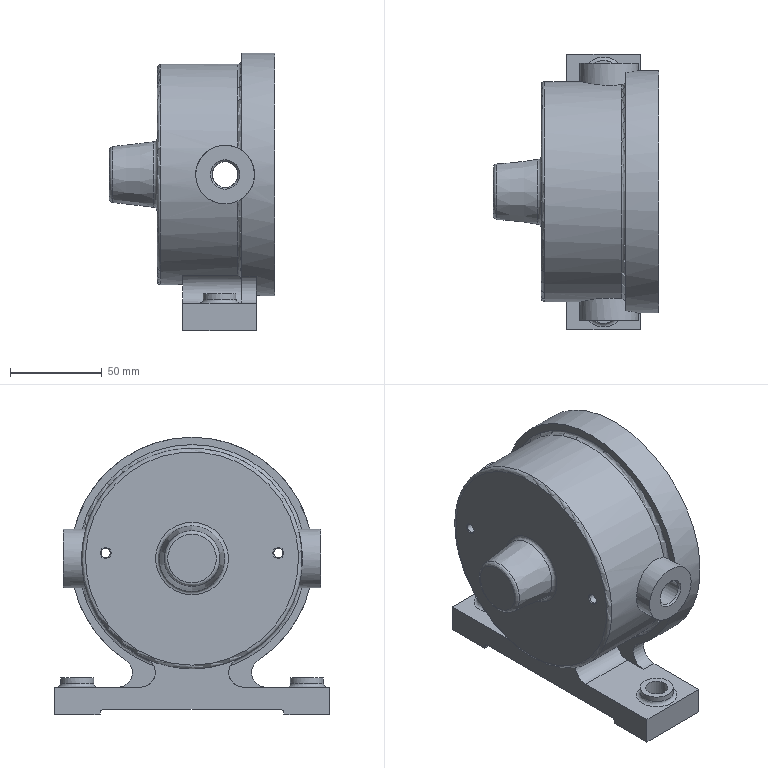Part | NX | features DATUM_CSYS 16, SKETCH 15, EXTRACT_FACE 11, EXTRUDE 10, HOLE PACKAGE 7, SIMPLE HOLE 7, SYMBOLIC_THREAD 7, Instance Feature 5, BLEND 3, Mirror Feature 3, EXTRACT_DATUM_AXIS 2, EXTRACT_DATUM_PLANE 2, EXTRACT_STRING 2, DATUM_AXIS 1, DATUM_PLANE 1, Pattern Feature 1, SWP104 1, UNITE 1 | 1 solid | 67 faces | box 90 x 150 x 151 mm | volume 479764 mm3 | cylinder 23 | plane 22 | cone 14 | torus 8 | commonest cylinder face diameters 5 x5 16 x4 14 x3 4 x2 12 x2 18 x2